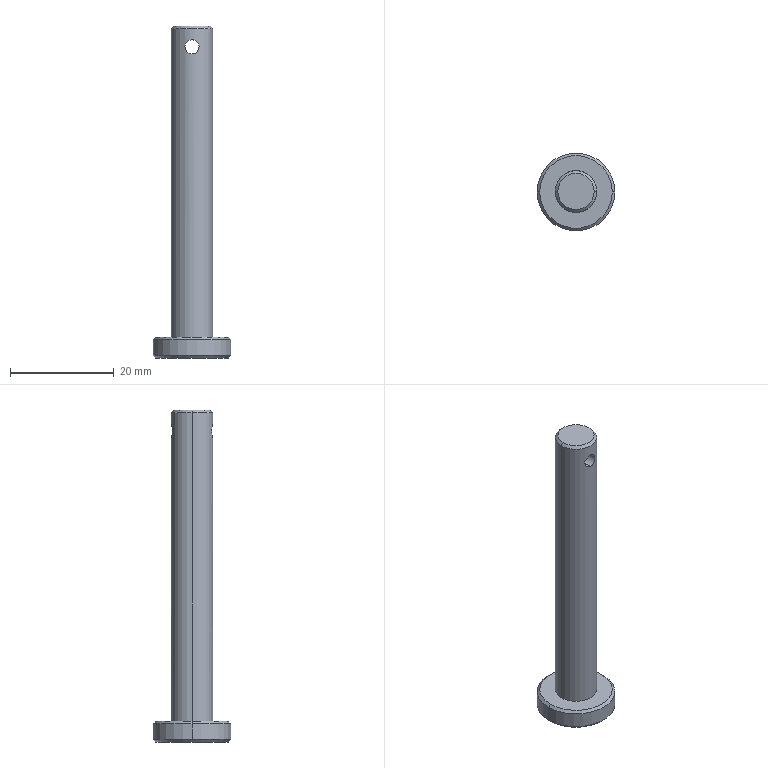Part | SolidWorks | features ICE 2, Chamfer 1, Extrusion 1 | 1 solid | 15 faces | box 15 x 15 x 64 mm | volume 3663 mm3 | cone 6 | cylinder 6 | plane 3 | commonest cylinder face diameters 2.7 x2 8 x2 15 x2
STEP:
#1=CARTESIAN_POINT('',(3.5,0.,60.));
#2=VERTEX_POINT('',#1);
#3=CARTESIAN_POINT('',(-3.5,0.,60.));
#4=VERTEX_POINT('',#3);
#5=CARTESIAN_POINT('',(0.,0.,60.));
#6=DIRECTION('',(0.,0.,1.));
#7=DIRECTION('',(1.,0.,0.));
#8=AXIS2_PLACEMENT_3D('',#5,#6,#7);
#9=CIRCLE('',#8,3.5);
#10=EDGE_CURVE('',#2,#4,#9,.T.);
#11=ORIENTED_EDGE('',*,*,#10,.F.);
#12=CARTESIAN_POINT('',(4.,0.,59.5));
#13=VERTEX_POINT('',#12);
#14=CARTESIAN_POINT('',(3.5,0.,60.));
#15=DIRECTION('',(0.7071,0.,-0.7071));
#16=VECTOR('',#15,1000.);
#17=LINE('',#14,#16);
#18=EDGE_CURVE('',#2,#13,#17,.T.);
#19=ORIENTED_EDGE('',*,*,#18,.T.);
#20=CARTESIAN_POINT('',(-4.,0.,59.5));
#21=VERTEX_POINT('',#20);
#22=CARTESIAN_POINT('',(0.,0.,59.5));
#23=DIRECTION('',(0.,0.,-1.));
#24=DIRECTION('',(1.,0.,0.));
#25=AXIS2_PLACEMENT_3D('',#22,#23,#24);
#26=CIRCLE('',#25,4.);
#27=EDGE_CURVE('',#21,#13,#26,.T.);
#28=ORIENTED_EDGE('',*,*,#27,.F.);
#29=CARTESIAN_POINT('',(-3.5,0.,60.));
#30=DIRECTION('',(-0.7071,0.,-0.7071));
#31=VECTOR('',#30,1000.);
#32=LINE('',#29,#31);
#33=EDGE_CURVE('',#4,#21,#32,.T.);
#34=ORIENTED_EDGE('',*,*,#33,.F.);
#35=EDGE_LOOP('',(#11,#19,#28,#34));
#36=FACE_OUTER_BOUND('',#35,.T.);
#37=CARTESIAN_POINT('',(0.,0.,60.));
#38=DIRECTION('',(0.,0.,-1.));
#39=DIRECTION('',(-1.,0.,0.));
#40=AXIS2_PLACEMENT_3D('',#37,#38,#39);
#41=CONICAL_SURFACE('',#40,3.5,0.7854);
#42=ADVANCED_FACE('',(#36),#41,.T.);
#43=CARTESIAN_POINT('',(7.,0.,0.));
#44=VERTEX_POINT('',#43);
#45=CARTESIAN_POINT('',(-7.,0.,0.));
#46=VERTEX_POINT('',#45);
#47=CARTESIAN_POINT('',(0.,0.,0.));
#48=DIRECTION('',(0.,0.,1.));
#49=DIRECTION('',(-1.,0.,0.));
#50=AXIS2_PLACEMENT_3D('',#47,#48,#49);
#51=CIRCLE('',#50,7.);
#52=EDGE_CURVE('',#44,#46,#51,.T.);
#53=ORIENTED_EDGE('',*,*,#52,.F.);
#54=CARTESIAN_POINT('',(7.5,0.,-0.5));
#55=VERTEX_POINT('',#54);
#56=CARTESIAN_POINT('',(7.5,0.,-0.5));
#57=DIRECTION('',(0.7071,0.,-0.7071));
#58=VECTOR('',#57,1000.);
#59=LINE('',#56,#58);
#60=EDGE_CURVE('',#44,#55,#59,.T.);
#61=ORIENTED_EDGE('',*,*,#60,.T.);
#62=CARTESIAN_POINT('',(-7.5,0.,-0.5));
#63=VERTEX_POINT('',#62);
#64=CARTESIAN_POINT('',(0.,0.,-0.5));
#65=DIRECTION('',(0.,0.,-1.));
#66=DIRECTION('',(-1.,0.,0.));
#67=AXIS2_PLACEMENT_3D('',#64,#65,#66);
#68=CIRCLE('',#67,7.5);
#69=EDGE_CURVE('',#63,#55,#68,.T.);
#70=ORIENTED_EDGE('',*,*,#69,.F.);
#71=CARTESIAN_POINT('',(-7.5,0.,-0.5));
#72=DIRECTION('',(-0.7071,0.,-0.7071));
#73=VECTOR('',#72,1000.);
#74=LINE('',#71,#73);
#75=EDGE_CURVE('',#46,#63,#74,.T.);
#76=ORIENTED_EDGE('',*,*,#75,.F.);
#77=EDGE_LOOP('',(#53,#61,#70,#76));
#78=FACE_OUTER_BOUND('',#77,.T.);
#79=CARTESIAN_POINT('',(0.,0.,-0.5));
#80=DIRECTION('',(0.,0.,-1.));
#81=DIRECTION('',(-1.,0.,0.));
#82=AXIS2_PLACEMENT_3D('',#79,#80,#81);
#83=CONICAL_SURFACE('',#82,7.5,0.7854);
#84=ADVANCED_FACE('',(#78),#83,.T.);
#85=CARTESIAN_POINT('',(-7.,0.,-4.));
#86=VERTEX_POINT('',#85);
#87=CARTESIAN_POINT('',(7.,0.,-4.));
#88=VERTEX_POINT('',#87);
#89=CARTESIAN_POINT('',(0.,0.,-4.));
#90=DIRECTION('',(0.,0.,-1.));
#91=DIRECTION('',(-1.,0.,0.));
#92=AXIS2_PLACEMENT_3D('',#89,#90,#91);
#93=CIRCLE('',#92,7.);
#94=EDGE_CURVE('',#86,#88,#93,.T.);
#95=ORIENTED_EDGE('',*,*,#94,.F.);
#96=CARTESIAN_POINT('',(-7.5,0.,-3.5));
#97=VERTEX_POINT('',#96);
#98=CARTESIAN_POINT('',(-7.,0.,-4.));
#99=DIRECTION('',(-0.7071,0.,0.7071));
#100=VECTOR('',#99,1000.);
#101=LINE('',#98,#100);
#102=EDGE_CURVE('',#86,#97,#101,.T.);
#103=ORIENTED_EDGE('',*,*,#102,.T.);
#104=CARTESIAN_POINT('',(7.5,0.,-3.5));
#105=VERTEX_POINT('',#104);
#106=CARTESIAN_POINT('',(0.,0.,-3.5));
#107=DIRECTION('',(0.,0.,1.));
#108=DIRECTION('',(-1.,0.,0.));
#109=AXIS2_PLACEMENT_3D('',#106,#107,#108);
#110=CIRCLE('',#109,7.5);
#111=EDGE_CURVE('',#105,#97,#110,.T.);
#112=ORIENTED_EDGE('',*,*,#111,.F.);
#113=CARTESIAN_POINT('',(7.,0.,-4.));
#114=DIRECTION('',(0.7071,0.,0.7071));
#115=VECTOR('',#114,1000.);
#116=LINE('',#113,#115);
#117=EDGE_CURVE('',#88,#105,#116,.T.);
#118=ORIENTED_EDGE('',*,*,#117,.F.);
#119=EDGE_LOOP('',(#95,#103,#112,#118));
#120=FACE_OUTER_BOUND('',#119,.T.);
#121=CARTESIAN_POINT('',(0.,0.,-4.));
#122=DIRECTION('',(0.,0.,1.));
#123=DIRECTION('',(1.,0.,0.));
#124=AXIS2_PLACEMENT_3D('',#121,#122,#123);
#125=CONICAL_SURFACE('',#124,7.,0.7854);
#126=ADVANCED_FACE('',(#120),#125,.T.);
#127=CARTESIAN_POINT('',(0.,-4.,54.65));
#128=VERTEX_POINT('',#127);
#129=CARTESIAN_POINT('',(0.,-4.,57.35));
#130=VERTEX_POINT('',#129);
#131=CARTESIAN_POINT('',(0.,-4.,54.65));
#132=CARTESIAN_POINT('',(-0.1771,-4.,54.65));
#133=CARTESIAN_POINT('',(-0.3558,-3.988,54.686));
#134=CARTESIAN_POINT('',(-0.6002,-3.956,54.788));
#135=CARTESIAN_POINT('',(-0.6792,-3.943,54.83));
#136=CARTESIAN_POINT('',(-0.8249,-3.915,54.928));
#137=CARTESIAN_POINT('',(-0.8925,-3.9,54.983));
#138=CARTESIAN_POINT('',(-1.079,-3.854,55.17));
#139=CARTESIAN_POINT('',(-1.178,-3.823,55.318));
#140=CARTESIAN_POINT('',(-1.281,-3.79,55.564));
#141=CARTESIAN_POINT('',(-1.306,-3.781,55.648));
#142=CARTESIAN_POINT('',(-1.341,-3.769,55.821));
#143=CARTESIAN_POINT('',(-1.35,-3.765,55.911));
#144=CARTESIAN_POINT('',(-1.35,-3.765,56.178));
#145=CARTESIAN_POINT('',(-1.314,-3.779,56.356));
#146=CARTESIAN_POINT('',(-1.179,-3.823,56.681));
#147=CARTESIAN_POINT('',(-1.078,-3.854,56.831));
#148=CARTESIAN_POINT('',(-0.8929,-3.9,57.016));
#149=CARTESIAN_POINT('',(-0.8239,-3.915,57.073));
#150=CARTESIAN_POINT('',(-0.6781,-3.943,57.171));
#151=CARTESIAN_POINT('',(-0.6009,-3.955,57.212));
#152=CARTESIAN_POINT('',(-0.4376,-3.977,57.28));
#153=CARTESIAN_POINT('',(-0.3516,-3.985,57.306));
#154=CARTESIAN_POINT('',(-0.1782,-3.997,57.341));
#155=CARTESIAN_POINT('',(-0.08989,-4.,57.35));
#156=CARTESIAN_POINT('',(0.,-4.,57.35));
#157=B_SPLINE_CURVE_WITH_KNOTS('',3,(#131,#132,#133,#134,#135,#136,#137,#138,#139,#140,#141,#142,#143,#144,#145,#146,#147,#148,#149,#150,#151,#152,#153,#154,#155,#156),.UNSPECIFIED.,.F.,.F.,(4,2,2,2,2,2,2,2,2,2,2,2,4),(0.004252,0.004784,0.005049,0.005315,0.005846,0.006112,0.006378,0.006909,0.007441,0.007706,0.007972,0.008238,0.008503),.UNSPECIFIED.);
#158=EDGE_CURVE('',#128,#130,#157,.T.);
#159=ORIENTED_EDGE('',*,*,#158,.F.);
#160=CARTESIAN_POINT('',(0.,4.,54.65));
#161=VERTEX_POINT('',#160);
#162=CARTESIAN_POINT('',(0.,-7.5,54.65));
#163=DIRECTION('',(0.,1.,0.));
#164=VECTOR('',#163,1000.);
#165=LINE('',#162,#164);
#166=EDGE_CURVE('',#128,#161,#165,.T.);
#167=ORIENTED_EDGE('',*,*,#166,.T.);
#168=CARTESIAN_POINT('',(0.,4.,57.35));
#169=VERTEX_POINT('',#168);
#170=CARTESIAN_POINT('',(0.,4.,57.35));
#171=CARTESIAN_POINT('',(-0.08991,4.,57.35));
#172=CARTESIAN_POINT('',(-0.1782,3.997,57.341));
#173=CARTESIAN_POINT('',(-0.3517,3.985,57.306));
#174=CARTESIAN_POINT('',(-0.4378,3.977,57.28));
#175=CARTESIAN_POINT('',(-0.6826,3.945,57.178));
#176=CARTESIAN_POINT('',(-0.8315,3.915,57.078));
#177=CARTESIAN_POINT('',(-1.079,3.854,56.831));
#178=CARTESIAN_POINT('',(-1.179,3.823,56.681));
#179=CARTESIAN_POINT('',(-1.314,3.779,56.357));
#180=CARTESIAN_POINT('',(-1.35,3.765,56.178));
#181=CARTESIAN_POINT('',(-1.35,3.765,55.912));
#182=CARTESIAN_POINT('',(-1.341,3.769,55.822));
#183=CARTESIAN_POINT('',(-1.306,3.781,55.648));
#184=CARTESIAN_POINT('',(-1.281,3.79,55.563));
#185=CARTESIAN_POINT('',(-1.178,3.823,55.317));
#186=CARTESIAN_POINT('',(-1.078,3.854,55.169));
#187=CARTESIAN_POINT('',(-0.8921,3.9,54.983));
#188=CARTESIAN_POINT('',(-0.8246,3.915,54.928));
#189=CARTESIAN_POINT('',(-0.6788,3.943,54.83));
#190=CARTESIAN_POINT('',(-0.5998,3.956,54.787));
#191=CARTESIAN_POINT('',(-0.3559,3.988,54.686));
#192=CARTESIAN_POINT('',(-0.1771,4.,54.65));
#193=CARTESIAN_POINT('',(0.,4.,54.65));
#194=B_SPLINE_CURVE_WITH_KNOTS('',3,(#170,#171,#172,#173,#174,#175,#176,#177,#178,#179,#180,#181,#182,#183,#184,#185,#186,#187,#188,#189,#190,#191,#192,#193),.UNSPECIFIED.,.F.,.F.,(4,2,2,2,2,2,2,2,2,2,2,4),(0.,0.0002658,0.0005315,0.001063,0.001595,0.002126,0.002392,0.002658,0.003189,0.003455,0.003721,0.004252),.UNSPECIFIED.);
#195=EDGE_CURVE('',#169,#161,#194,.T.);
#196=ORIENTED_EDGE('',*,*,#195,.F.);
#197=CARTESIAN_POINT('',(0.,-7.5,57.35));
#198=DIRECTION('',(0.,1.,0.));
#199=VECTOR('',#198,1000.);
#200=LINE('',#197,#199);
#201=EDGE_CURVE('',#130,#169,#200,.T.);
#202=ORIENTED_EDGE('',*,*,#201,.F.);
#203=EDGE_LOOP('',(#159,#167,#196,#202));
#204=FACE_OUTER_BOUND('',#203,.T.);
#205=CARTESIAN_POINT('',(0.,-7.5,56.));
#206=DIRECTION('',(0.,1.,0.));
#207=DIRECTION('',(0.,0.,1.));
#208=AXIS2_PLACEMENT_3D('',#205,#206,#207);
#209=CYLINDRICAL_SURFACE('',#208,1.35);
#210=ADVANCED_FACE('',(#204),#209,.F.);
#211=ORIENTED_EDGE('',*,*,#111,.T.);
#212=CARTESIAN_POINT('',(-7.5,0.,-4.));
#213=DIRECTION('',(0.,0.,1.));
#214=VECTOR('',#213,1000.);
#215=LINE('',#212,#214);
#216=EDGE_CURVE('',#97,#63,#215,.T.);
#217=ORIENTED_EDGE('',*,*,#216,.T.);
#218=ORIENTED_EDGE('',*,*,#69,.T.);
#219=CARTESIAN_POINT('',(7.5,0.,-4.));
#220=DIRECTION('',(0.,0.,1.));
#221=VECTOR('',#220,1000.);
#222=LINE('',#219,#221);
#223=EDGE_CURVE('',#105,#55,#222,.T.);
#224=ORIENTED_EDGE('',*,*,#223,.F.);
#225=EDGE_LOOP('',(#211,#217,#218,#224));
#226=FACE_OUTER_BOUND('',#225,.T.);
#227=CARTESIAN_POINT('',(0.,0.,-4.));
#228=DIRECTION('',(0.,0.,1.));
#229=DIRECTION('',(1.,0.,0.));
#230=AXIS2_PLACEMENT_3D('',#227,#228,#229);
#231=CYLINDRICAL_SURFACE('',#230,7.5);
#232=ADVANCED_FACE('',(#226),#231,.T.);
#233=ORIENTED_EDGE('',*,*,#195,.T.);
#234=CARTESIAN_POINT('',(0.,4.,54.65));
#235=CARTESIAN_POINT('',(0.1771,4.,54.65));
#236=CARTESIAN_POINT('',(0.3558,3.988,54.686));
#237=CARTESIAN_POINT('',(0.6002,3.956,54.788));
#238=CARTESIAN_POINT('',(0.6792,3.943,54.83));
#239=CARTESIAN_POINT('',(0.8249,3.915,54.928));
#240=CARTESIAN_POINT('',(0.8925,3.9,54.983));
#241=CARTESIAN_POINT('',(1.079,3.854,55.17));
#242=CARTESIAN_POINT('',(1.178,3.823,55.318));
#243=CARTESIAN_POINT('',(1.281,3.79,55.564));
#244=CARTESIAN_POINT('',(1.306,3.781,55.648));
#245=CARTESIAN_POINT('',(1.341,3.769,55.821));
#246=CARTESIAN_POINT('',(1.35,3.765,55.911));
#247=CARTESIAN_POINT('',(1.35,3.765,56.178));
#248=CARTESIAN_POINT('',(1.314,3.779,56.356));
#249=CARTESIAN_POINT('',(1.179,3.823,56.681));
#250=CARTESIAN_POINT('',(1.078,3.854,56.831));
#251=CARTESIAN_POINT('',(0.8929,3.9,57.016));
#252=CARTESIAN_POINT('',(0.8239,3.915,57.073));
#253=CARTESIAN_POINT('',(0.6781,3.943,57.171));
#254=CARTESIAN_POINT('',(0.6009,3.955,57.212));
#255=CARTESIAN_POINT('',(0.4376,3.977,57.28));
#256=CARTESIAN_POINT('',(0.3516,3.985,57.306));
#257=CARTESIAN_POINT('',(0.1782,3.997,57.341));
#258=CARTESIAN_POINT('',(0.08989,4.,57.35));
#259=CARTESIAN_POINT('',(0.,4.,57.35));
#260=B_SPLINE_CURVE_WITH_KNOTS('',3,(#234,#235,#236,#237,#238,#239,#240,#241,#242,#243,#244,#245,#246,#247,#248,#249,#250,#251,#252,#253,#254,#255,#256,#257,#258,#259),.UNSPECIFIED.,.F.,.F.,(4,2,2,2,2,2,2,2,2,2,2,2,4),(0.004252,0.004784,0.005049,0.005315,0.005846,0.006112,0.006378,0.006909,0.007441,0.007706,0.007972,0.008238,0.008503),.UNSPECIFIED.);
#261=EDGE_CURVE('',#161,#169,#260,.T.);
#262=ORIENTED_EDGE('',*,*,#261,.T.);
#263=EDGE_LOOP('',(#233,#262));
#264=FACE_BOUND('',#263,.T.);
#265=ORIENTED_EDGE('',*,*,#27,.T.);
#266=CARTESIAN_POINT('',(4.,0.,0.));
#267=VERTEX_POINT('',#266);
#268=CARTESIAN_POINT('',(4.,0.,60.));
#269=DIRECTION('',(0.,0.,-1.));
#270=VECTOR('',#269,1000.);
#271=LINE('',#268,#270);
#272=EDGE_CURVE('',#13,#267,#271,.T.);
#273=ORIENTED_EDGE('',*,*,#272,.T.);
#274=CARTESIAN_POINT('',(-4.,0.,0.));
#275=VERTEX_POINT('',#274);
#276=CARTESIAN_POINT('',(0.,0.,0.));
#277=DIRECTION('',(0.,0.,1.));
#278=DIRECTION('',(1.,0.,0.));
#279=AXIS2_PLACEMENT_3D('',#276,#277,#278);
#280=CIRCLE('',#279,4.);
#281=EDGE_CURVE('',#267,#275,#280,.T.);
#282=ORIENTED_EDGE('',*,*,#281,.T.);
#283=CARTESIAN_POINT('',(-4.,0.,60.));
#284=DIRECTION('',(0.,0.,-1.));
#285=VECTOR('',#284,1000.);
#286=LINE('',#283,#285);
#287=EDGE_CURVE('',#21,#275,#286,.T.);
#288=ORIENTED_EDGE('',*,*,#287,.F.);
#289=EDGE_LOOP('',(#265,#273,#282,#288));
#290=FACE_OUTER_BOUND('',#289,.T.);
#291=CARTESIAN_POINT('',(0.,0.,60.));
#292=DIRECTION('',(0.,0.,-1.));
#293=DIRECTION('',(-1.,0.,0.));
#294=AXIS2_PLACEMENT_3D('',#291,#292,#293);
#295=CYLINDRICAL_SURFACE('',#294,4.);
#296=ADVANCED_FACE('',(#264,#290),#295,.T.);
#297=ORIENTED_EDGE('',*,*,#272,.F.);
#298=CARTESIAN_POINT('',(0.,0.,59.5));
#299=DIRECTION('',(0.,0.,-1.));
#300=DIRECTION('',(1.,0.,0.));
#301=AXIS2_PLACEMENT_3D('',#298,#299,#300);
#302=CIRCLE('',#301,4.);
#303=EDGE_CURVE('',#13,#21,#302,.T.);
#304=ORIENTED_EDGE('',*,*,#303,.T.);
#305=ORIENTED_EDGE('',*,*,#287,.T.);
#306=CARTESIAN_POINT('',(0.,0.,0.));
#307=DIRECTION('',(0.,0.,1.));
#308=DIRECTION('',(1.,0.,0.));
#309=AXIS2_PLACEMENT_3D('',#306,#307,#308);
#310=CIRCLE('',#309,4.);
#311=EDGE_CURVE('',#275,#267,#310,.T.);
#312=ORIENTED_EDGE('',*,*,#311,.T.);
#313=EDGE_LOOP('',(#297,#304,#305,#312));
#314=FACE_OUTER_BOUND('',#313,.T.);
#315=CARTESIAN_POINT('',(0.,-4.,57.35));
#316=CARTESIAN_POINT('',(0.08991,-4.,57.35));
#317=CARTESIAN_POINT('',(0.1782,-3.997,57.341));
#318=CARTESIAN_POINT('',(0.3517,-3.985,57.306));
#319=CARTESIAN_POINT('',(0.4378,-3.977,57.28));
#320=CARTESIAN_POINT('',(0.6826,-3.945,57.178));
#321=CARTESIAN_POINT('',(0.8315,-3.915,57.078));
#322=CARTESIAN_POINT('',(1.079,-3.854,56.831));
#323=CARTESIAN_POINT('',(1.179,-3.823,56.681));
#324=CARTESIAN_POINT('',(1.314,-3.779,56.357));
#325=CARTESIAN_POINT('',(1.35,-3.765,56.178));
#326=CARTESIAN_POINT('',(1.35,-3.765,55.912));
#327=CARTESIAN_POINT('',(1.341,-3.769,55.822));
#328=CARTESIAN_POINT('',(1.306,-3.781,55.648));
#329=CARTESIAN_POINT('',(1.281,-3.79,55.563));
#330=CARTESIAN_POINT('',(1.178,-3.823,55.317));
#331=CARTESIAN_POINT('',(1.078,-3.854,55.169));
#332=CARTESIAN_POINT('',(0.8921,-3.9,54.983));
#333=CARTESIAN_POINT('',(0.8246,-3.915,54.928));
#334=CARTESIAN_POINT('',(0.6788,-3.943,54.83));
#335=CARTESIAN_POINT('',(0.5998,-3.956,54.787));
#336=CARTESIAN_POINT('',(0.3559,-3.988,54.686));
#337=CARTESIAN_POINT('',(0.1771,-4.,54.65));
#338=CARTESIAN_POINT('',(0.,-4.,54.65));
#339=B_SPLINE_CURVE_WITH_KNOTS('',3,(#315,#316,#317,#318,#319,#320,#321,#322,#323,#324,#325,#326,#327,#328,#329,#330,#331,#332,#333,#334,#335,#336,#337,#338),.UNSPECIFIED.,.F.,.F.,(4,2,2,2,2,2,2,2,2,2,2,4),(0.,0.0002658,0.0005315,0.001063,0.001595,0.002126,0.002392,0.002658,0.003189,0.003455,0.003721,0.004252),.UNSPECIFIED.);
#340=EDGE_CURVE('',#130,#128,#339,.T.);
#341=ORIENTED_EDGE('',*,*,#340,.T.);
#342=ORIENTED_EDGE('',*,*,#158,.T.);
#343=EDGE_LOOP('',(#341,#342));
#344=FACE_BOUND('',#343,.T.);
#345=CARTESIAN_POINT('',(0.,0.,60.));
#346=DIRECTION('',(0.,0.,-1.));
#347=DIRECTION('',(-1.,0.,0.));
#348=AXIS2_PLACEMENT_3D('',#345,#346,#347);
#349=CYLINDRICAL_SURFACE('',#348,4.);
#350=ADVANCED_FACE('',(#314,#344),#349,.T.);
#351=CARTESIAN_POINT('',(0.,0.,60.));
#352=DIRECTION('',(0.,0.,1.));
#353=DIRECTION('',(1.,0.,0.));
#354=AXIS2_PLACEMENT_3D('',#351,#352,#353);
#355=CIRCLE('',#354,3.5);
#356=EDGE_CURVE('',#4,#2,#355,.T.);
#357=ORIENTED_EDGE('',*,*,#356,.T.);
#358=ORIENTED_EDGE('',*,*,#10,.T.);
#359=EDGE_LOOP('',(#357,#358));
#360=FACE_OUTER_BOUND('',#359,.T.);
#361=CARTESIAN_POINT('',(0.,0.,60.));
#362=DIRECTION('',(0.,0.,1.));
#363=DIRECTION('',(1.,0.,0.));
#364=AXIS2_PLACEMENT_3D('',#361,#362,#363);
#365=PLANE('',#364);
#366=ADVANCED_FACE('',(#360),#365,.T.);
#367=ORIENTED_EDGE('',*,*,#216,.F.);
#368=CARTESIAN_POINT('',(0.,0.,-3.5));
#369=DIRECTION('',(0.,0.,1.));
#370=DIRECTION('',(-1.,0.,0.));
#371=AXIS2_PLACEMENT_3D('',#368,#369,#370);
#372=CIRCLE('',#371,7.5);
#373=EDGE_CURVE('',#97,#105,#372,.T.);
#374=ORIENTED_EDGE('',*,*,#373,.T.);
#375=ORIENTED_EDGE('',*,*,#223,.T.);
#376=CARTESIAN_POINT('',(0.,0.,-0.5));
#377=DIRECTION('',(0.,0.,-1.));
#378=DIRECTION('',(-1.,0.,0.));
#379=AXIS2_PLACEMENT_3D('',#376,#377,#378);
#380=CIRCLE('',#379,7.5);
#381=EDGE_CURVE('',#55,#63,#380,.T.);
#382=ORIENTED_EDGE('',*,*,#381,.T.);
#383=EDGE_LOOP('',(#367,#374,#375,#382));
#384=FACE_OUTER_BOUND('',#383,.T.);
#385=CARTESIAN_POINT('',(0.,0.,-4.));
#386=DIRECTION('',(0.,0.,1.));
#387=DIRECTION('',(1.,0.,0.));
#388=AXIS2_PLACEMENT_3D('',#385,#386,#387);
#389=CYLINDRICAL_SURFACE('',#388,7.5);
#390=ADVANCED_FACE('',(#384),#389,.T.);
#391=CARTESIAN_POINT('',(0.,0.,-4.));
#392=DIRECTION('',(0.,0.,-1.));
#393=DIRECTION('',(-1.,0.,0.));
#394=AXIS2_PLACEMENT_3D('',#391,#392,#393);
#395=CIRCLE('',#394,7.);
#396=EDGE_CURVE('',#88,#86,#395,.T.);
#397=ORIENTED_EDGE('',*,*,#396,.T.);
#398=ORIENTED_EDGE('',*,*,#94,.T.);
#399=EDGE_LOOP('',(#397,#398));
#400=FACE_OUTER_BOUND('',#399,.T.);
#401=CARTESIAN_POINT('',(0.,0.,-4.));
#402=DIRECTION('',(0.,0.,-1.));
#403=DIRECTION('',(-1.,0.,0.));
#404=AXIS2_PLACEMENT_3D('',#401,#402,#403);
#405=PLANE('',#404);
#406=ADVANCED_FACE('',(#400),#405,.T.);
#407=CARTESIAN_POINT('',(0.,0.,0.));
#408=DIRECTION('',(0.,0.,1.));
#409=DIRECTION('',(-1.,0.,0.));
#410=AXIS2_PLACEMENT_3D('',#407,#408,#409);
#411=CIRCLE('',#410,7.);
#412=EDGE_CURVE('',#46,#44,#411,.T.);
#413=ORIENTED_EDGE('',*,*,#412,.T.);
#414=ORIENTED_EDGE('',*,*,#52,.T.);
#415=EDGE_LOOP('',(#413,#414));
#416=FACE_OUTER_BOUND('',#415,.T.);
#417=ORIENTED_EDGE('',*,*,#311,.F.);
#418=ORIENTED_EDGE('',*,*,#281,.F.);
#419=EDGE_LOOP('',(#417,#418));
#420=FACE_BOUND('',#419,.T.);
#421=CARTESIAN_POINT('',(0.,0.,0.));
#422=DIRECTION('',(0.,0.,-1.));
#423=DIRECTION('',(-1.,0.,0.));
#424=AXIS2_PLACEMENT_3D('',#421,#422,#423);
#425=PLANE('',#424);
#426=ADVANCED_FACE('',(#416,#420),#425,.F.);
#427=ORIENTED_EDGE('',*,*,#166,.F.);
#428=ORIENTED_EDGE('',*,*,#340,.F.);
#429=ORIENTED_EDGE('',*,*,#201,.T.);
#430=ORIENTED_EDGE('',*,*,#261,.F.);
#431=EDGE_LOOP('',(#427,#428,#429,#430));
#432=FACE_OUTER_BOUND('',#431,.T.);
#433=CARTESIAN_POINT('',(0.,-7.5,56.));
#434=DIRECTION('',(0.,1.,0.));
#435=DIRECTION('',(0.,0.,1.));
#436=AXIS2_PLACEMENT_3D('',#433,#434,#435);
#437=CYLINDRICAL_SURFACE('',#436,1.35);
#438=ADVANCED_FACE('',(#432),#437,.F.);
#439=ORIENTED_EDGE('',*,*,#102,.F.);
#440=ORIENTED_EDGE('',*,*,#396,.F.);
#441=ORIENTED_EDGE('',*,*,#117,.T.);
#442=ORIENTED_EDGE('',*,*,#373,.F.);
#443=EDGE_LOOP('',(#439,#440,#441,#442));
#444=FACE_OUTER_BOUND('',#443,.T.);
#445=CARTESIAN_POINT('',(0.,0.,-4.));
#446=DIRECTION('',(0.,0.,1.));
#447=DIRECTION('',(1.,0.,0.));
#448=AXIS2_PLACEMENT_3D('',#445,#446,#447);
#449=CONICAL_SURFACE('',#448,7.,0.7854);
#450=ADVANCED_FACE('',(#444),#449,.T.);
#451=ORIENTED_EDGE('',*,*,#60,.F.);
#452=ORIENTED_EDGE('',*,*,#412,.F.);
#453=ORIENTED_EDGE('',*,*,#75,.T.);
#454=ORIENTED_EDGE('',*,*,#381,.F.);
#455=EDGE_LOOP('',(#451,#452,#453,#454));
#456=FACE_OUTER_BOUND('',#455,.T.);
#457=CARTESIAN_POINT('',(0.,0.,-0.5));
#458=DIRECTION('',(0.,0.,-1.));
#459=DIRECTION('',(-1.,0.,0.));
#460=AXIS2_PLACEMENT_3D('',#457,#458,#459);
#461=CONICAL_SURFACE('',#460,7.5,0.7854);
#462=ADVANCED_FACE('',(#456),#461,.T.);
#463=ORIENTED_EDGE('',*,*,#18,.F.);
#464=ORIENTED_EDGE('',*,*,#356,.F.);
#465=ORIENTED_EDGE('',*,*,#33,.T.);
#466=ORIENTED_EDGE('',*,*,#303,.F.);
#467=EDGE_LOOP('',(#463,#464,#465,#466));
#468=FACE_OUTER_BOUND('',#467,.T.);
#469=CARTESIAN_POINT('',(0.,0.,60.));
#470=DIRECTION('',(0.,0.,-1.));
#471=DIRECTION('',(-1.,0.,0.));
#472=AXIS2_PLACEMENT_3D('',#469,#470,#471);
#473=CONICAL_SURFACE('',#472,3.5,0.7854);
#474=ADVANCED_FACE('',(#468),#473,.T.);
#475=CLOSED_SHELL('',(#42,#84,#126,#210,#232,#296,#350,#366,#390,#406,#426,#438,#450,#462,#474));
#476=MANIFOLD_SOLID_BREP('',#475);
#477=CARTESIAN_POINT('',(0.,0.,0.));
#478=DIRECTION('',(0.,0.,1.));
#479=DIRECTION('',(1.,0.,0.));
#480=AXIS2_PLACEMENT_3D('',#477,#478,#479);
#481=(LENGTH_UNIT()NAMED_UNIT(*)SI_UNIT(.MILLI.,.METRE.));
#482=UNCERTAINTY_MEASURE_WITH_UNIT(LENGTH_MEASURE(0.00001),#481,'','');
#483=(NAMED_UNIT(*)PLANE_ANGLE_UNIT()SI_UNIT($,.RADIAN.));
#484=(NAMED_UNIT(*)SI_UNIT($,.STERADIAN.)SOLID_ANGLE_UNIT());
#485=(GEOMETRIC_REPRESENTATION_CONTEXT(3)GLOBAL_UNCERTAINTY_ASSIGNED_CONTEXT((#482))GLOBAL_UNIT_ASSIGNED_CONTEXT((#481,#483,#484))REPRESENTATION_CONTEXT('',''));
#486=ADVANCED_BREP_SHAPE_REPRESENTATION('',(#476,#480),#485);